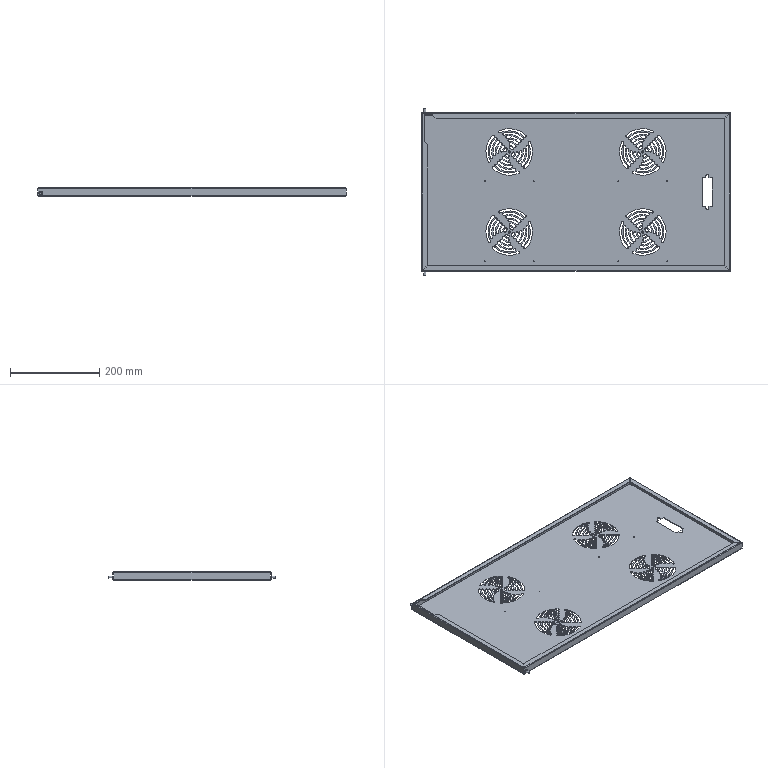Part | STEP file | FHD-021-004-A rear door A | 1 solid | 500 faces | box 693 x 376 x 18 mm | volume 424515 mm3 | cylinder 417 | plane 71 | spline 12 | commonest cylinder face diameters 5 x198 15 x16 25 x16 31 x16 41 x16 47 x16